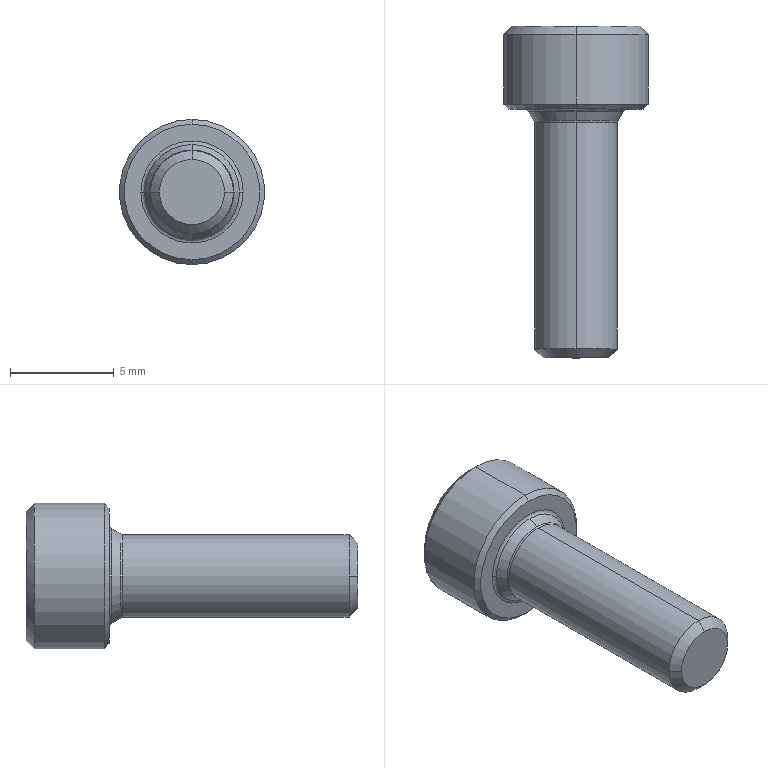Part | STEP file | 1 solid | 44 faces | box 7 x 16 x 7 mm | volume 280.848 mm3 | cone 19 | plane 15 | cylinder 6 | spline 4 | commonest cylinder face diameters 3 x2 4 x2 7 x2